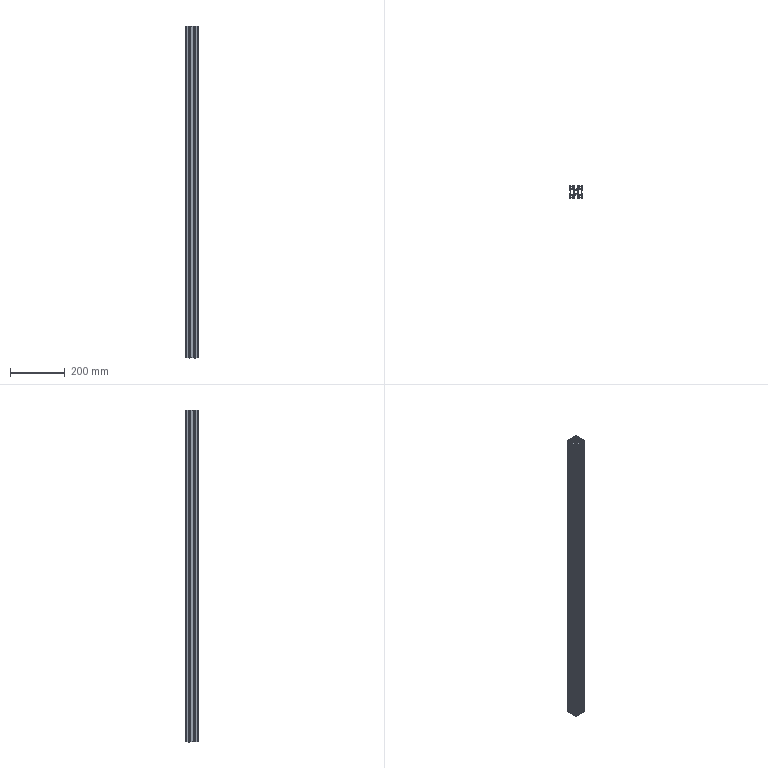Part | STEP file | 4545-1210 aluminium profile (upper cross long) | 1 solid | 262 faces | box 45 x 45 x 1210 mm | volume 839555 mm3 | plane 186 | cylinder 76 | commonest cylinder face diameters 2 x44 8 x20 12 x8 4 x4